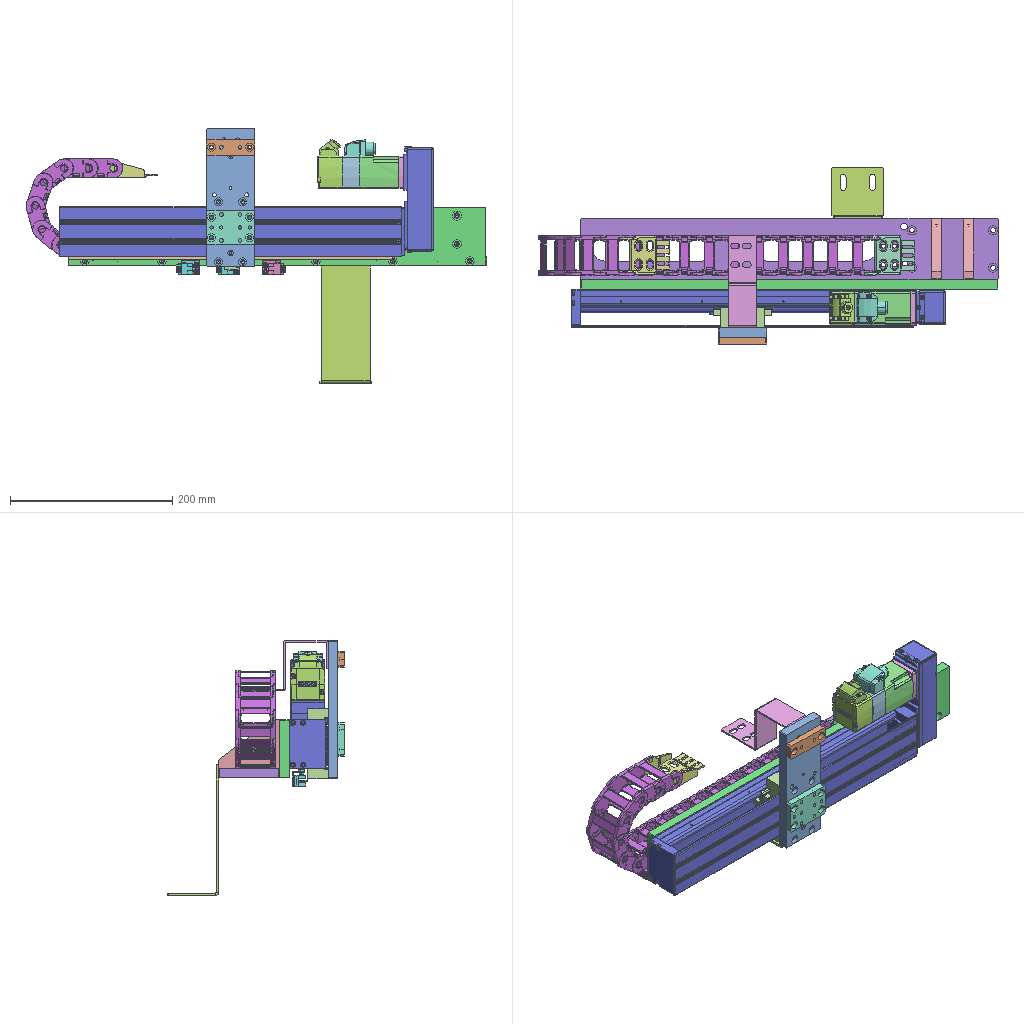Assembly | SolidWorks | 29 different items | 48 placed | box 567 x 218 x 314 mm
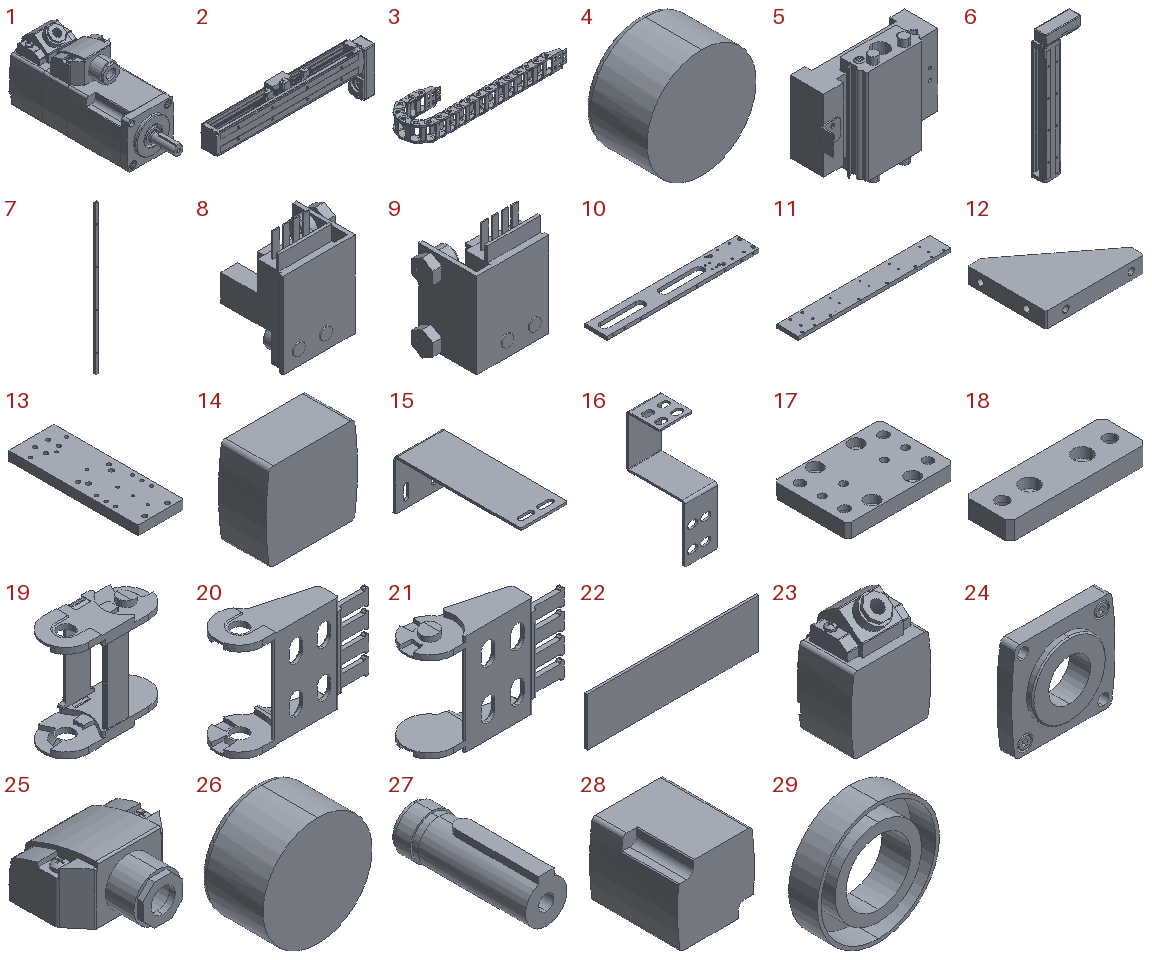Parts list (item | name | quantity | parent item | size | volume | features):
1 | (subassembly) | x1 | - | 42.009 x 131.188 x 60.7 mm | 192000 mm3 | -
2 | (subassembly) | x1 | - | 461 x 48 x 158.3 mm | 640236 mm3 | -
3 | (subassembly) | x1 | - | - | 173847 mm3 | -
4 | - | x1 | in 1 | 5.232 x 3 x 5.232 mm | 54.683 mm3 | features BaseBody 1
5 | - | x1 | in 2 | 89.2 x 36 x 82.5 mm | 126325 mm3 | features BaseBody 1
6 | - | x1 | in 2 | 136.45 x 47 x 461 mm | 496901 mm3 | features BaseBody 2
7 | - | x1 | in 2 | 8 x 5 x 400 mm | 7551 mm3 | features BaseBody 1
8 | - | x1 | in 2 | 21.6 x 16.9 x 28.375 mm | 3154 mm3 | features BaseBody 1
9 | - | x2 | in 2 | 21.6 x 16.9 x 28.375 mm | 3154 mm3 | features BaseBody 1
10 | - | x1 | - | 515 x 75 x 12 mm | 349062 mm3 | features HoleWzd 7, Chamfer 1, Extrusion 1, ICE 1
11 | - | x1 | - | 515 x 72 x 12 mm | 434783 mm3 | features HoleWzd 5, Chamfer 1, Extrusion 1
12 | - | x2 | - | 75 x 60 x 12 mm | 33384 mm3 | features HoleWzd 2, Chamfer 1, Extrusion 1, ICE 1
13 | - | x1 | - | 60 x 170.4 x 12 mm | 116995 mm3 | features HoleWzd 6, Chamfer 1, Cut 1, Extrusion 1
14 | - | x1 | in 1 | 42.009 x 21.95 x 40 mm | 35954 mm3 | features BaseBody 1
15 | - | x1 | - | 64 x 162 x 63 mm | 38960 mm3 | features HoleWzd 2, Chamfer 1, EdgeFlange 1, FlatPattern 1, SMBaseFlange 1, SheetMetal 1
16 | - | x1 | - | 35 x 62 x 114 mm | 13287 mm3 | features EdgeFlange 3, HoleWzd 2, Chamfer 1, FlatPattern 1, SMBaseFlange 1, SheetMetal 1
17 | - | x1 | - | 60 x 42 x 8 mm | 16637 mm3 | features HoleWzd 2, ICE 2, Chamfer 1, Extrusion 1
18 | - | x1 | - | 60 x 20 x 8 mm | 8007 mm3 | features HoleWzd 2, Chamfer 1, Extrusion 1
19 | - | x18 | in 3 | 53.492 x 23 x 49.2 mm | 8720 mm3 | features BaseBody 1
20 | - | x1 | in 3 | 66.5 x 23 x 49.2 mm | 8263 mm3 | features BaseBody 1
21 | - | x1 | in 3 | 66.5 x 23 x 49.2 mm | 8628 mm3 | features BaseBody 1
22 | - | x1 | in 1 | 21.7 x 0.588 x 6.16 mm | 55.825 mm3 | features BaseBody 1
23 | - | x1 | in 1 | 42.009 x 30.001 x 60.7 mm | 55286 mm3 | features BaseBody 1
24 | - | x1 | in 1 | 42.009 x 8.51 x 40 mm | 9357 mm3 | features BaseBody 1
25 | - | x1 | in 1 | 36 x 38.3 x 19.99 mm | 14358 mm3 | features BaseBody 1
26 | - | x1 | in 1 | 5.232 x 3 x 5.232 mm | 54.683 mm3 | features BaseBody 1
27 | - | x1 | in 1 | 8.5 x 25.7 x 9.25 mm | 1306 mm3 | features BaseBody 1
28 | - | x1 | in 1 | 42.009 x 48 x 40 mm | 75232 mm3 | features BaseBody 1
29 | - | x1 | in 1 | 16.96 x 4 x 16.96 mm | 341.308 mm3 | features BaseBody 1
Mates (type | each side: item.copy, entity, surface, feature):
Concentric | 27.1 face cylinder Input1 | 6.1 face cylinder Input1
Coincident | 24.1 face plane Input1 | 6.1 face plane Input2
Parallel | 24.1 face plane Input1 | 6.1 face plane Input2
Coincident | 10.1 face plane Boss-Extrude1 | 20.1 face plane Input1
DistanceDim | 20.1 face plane Input1 | 11.1 face plane Boss-Extrude1
DistanceDim | 20.1 face plane Input1 | 10.1 face plane Boss-Extrude1
Coincident | 10.1 face plane Boss-Extrude1 | 6.1 face plane Input2
Coincident | 13.1 face plane Boss-Extrude1 | 5.1 face plane Input1 | 2 times
Width | 5.1 face plane Input1 | 5.1 face plane Input1 | 13.1 face plane Boss-Extrude1 | 13.1 face plane Boss-Extrude1
DistanceDim | 6.1 face plane Input2 | 11.1 face plane Boss-Extrude1
Coincident | 6.1 face plane Input2 | 11.1 face plane Boss-Extrude1
Coincident | 10.1 face plane Boss-Extrude1 | 11.1 face plane Boss-Extrude1 | 3 times
Coincident | 10.1 face plane Boss-Extrude1 | 15.1 face plane Base-Flange1
DistanceDim | 15.1 plane | 10.1 face plane Boss-Extrude1
DistanceDim | 15.1 face plane Base-Flange1 | 10.1 face plane Boss-Extrude1
Coincident | 10.1 face plane Boss-Extrude1 | 12.1 face plane Boss-Extrude1
Coincident | 10.1 face plane Boss-Extrude1 | 12.2 face plane Boss-Extrude1
DistanceDim | 12.2 face plane Boss-Extrude1 | 10.1 face plane Boss-Extrude1
DistanceDim | 12.1 face plane Boss-Extrude1 | 10.1 face plane Boss-Extrude1
Coincident | 11.1 face plane Boss-Extrude1 | 12.1 face plane Boss-Extrude1
Coincident | 11.1 face plane Boss-Extrude1 | 12.2 face plane Boss-Extrude1
Coincident | 13.1 face plane Boss-Extrude1 | 16.1 face plane Base-Flange1
Width | 16.1 face plane Base-Flange1 | 16.1 face plane Base-Flange1 | 13.1 face plane Boss-Extrude1 | 13.1 face plane Boss-Extrude1
Coincident | 13.1 face plane Boss-Extrude1 | 16.1 face plane Edge-Flange1
Coincident | 13.1 face plane Boss-Extrude1 | 17.1 face plane Boss-Extrude1
Concentric | 13.1 face cylinder M5 Tapped Hole1 | 17.1 face cylinder CBORE for M5 Hex Socket Head Cap Screw1